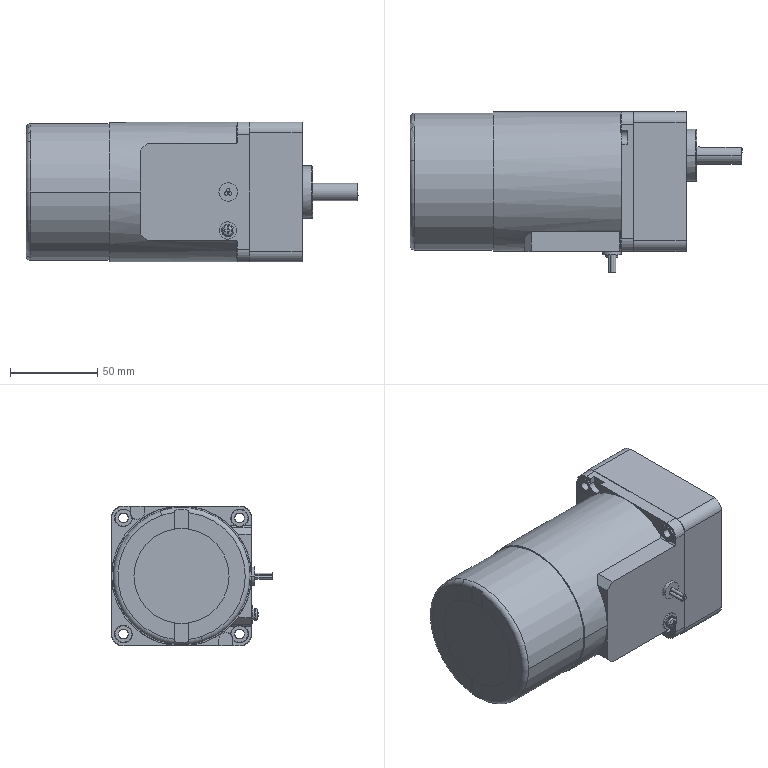Part | SolidWorks | features BaseBody 2 | 2 solids | 178 faces | box 190 x 92 x 80 mm | volume 778868 mm3 | plane 90 | cylinder 69 | torus 14 | cone 3 | sphere 2 | commonest cylinder face diameters 5.5 x16 10 x10 2 x8 4 x5 12 x4 14.6 x4